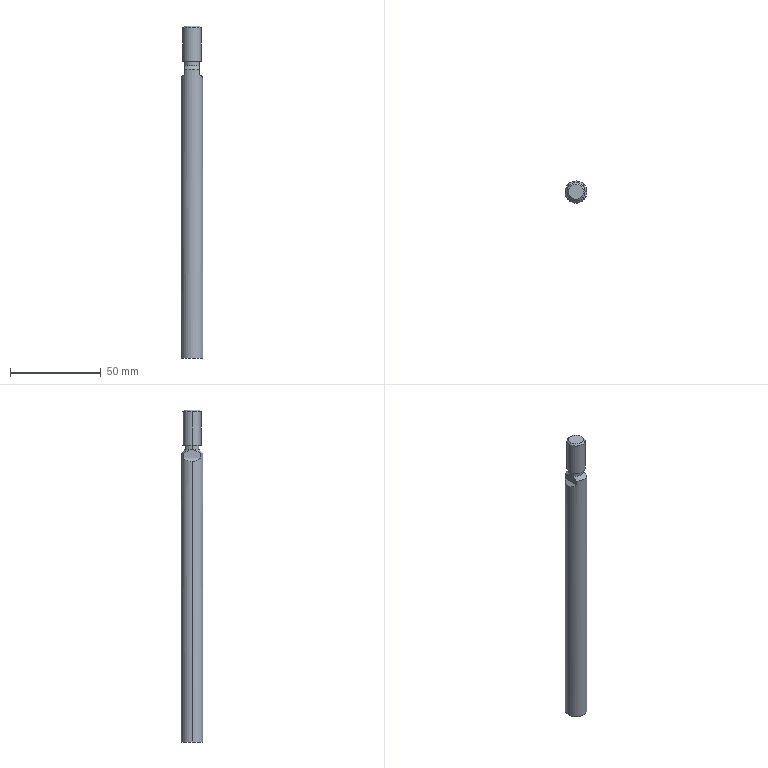Part | STEP file | rod_A_CDM2B32_150_C76_0_ | 1 solid | 19 faces | box 12 x 12 x 183 mm | volume 19693 mm3 | plane 9 | cylinder 6 | cone 4 | commonest cylinder face diameters 8.16 x2 10 x2 12 x2
STEP:
#1=CARTESIAN_POINT('',(6.,0.,-151.));
#2=VERTEX_POINT('',#1);
#3=CARTESIAN_POINT('',(-6.,0.,-151.));
#4=VERTEX_POINT('',#3);
#5=CARTESIAN_POINT('',(0.,0.,-151.));
#6=DIRECTION('',(0.,0.,1.));
#7=DIRECTION('',(1.,0.,0.));
#8=AXIS2_PLACEMENT_3D('',#5,#6,#7);
#9=CIRCLE('',#8,6.);
#10=EDGE_CURVE('',#2,#4,#9,.T.);
#11=ORIENTED_EDGE('',*,*,#10,.T.);
#12=CARTESIAN_POINT('',(-6.,0.,3.5));
#13=VERTEX_POINT('',#12);
#14=CARTESIAN_POINT('',(-6.,0.,-151.));
#15=DIRECTION('',(0.,0.,1.));
#16=VECTOR('',#15,1000.);
#17=LINE('',#14,#16);
#18=EDGE_CURVE('',#4,#13,#17,.T.);
#19=ORIENTED_EDGE('',*,*,#18,.T.);
#20=CARTESIAN_POINT('',(-4.,4.472,5.5));
#21=VERTEX_POINT('',#20);
#22=CARTESIAN_POINT('',(-6.,0.,3.5));
#23=CARTESIAN_POINT('',(-6.,1.734,3.5));
#24=CARTESIAN_POINT('',(-5.292,3.316,4.208));
#25=CARTESIAN_POINT('',(-4.,4.472,5.5));
#26=(BOUNDED_CURVE()B_SPLINE_CURVE(3,(#22,#23,#24,#25),.UNSPECIFIED.,.F.,.F.)B_SPLINE_CURVE_WITH_KNOTS((4,4),(3.142,3.983),.UNSPECIFIED.)CURVE()GEOMETRIC_REPRESENTATION_ITEM()RATIONAL_B_SPLINE_CURVE((1.,0.9419,0.9419,1.))REPRESENTATION_ITEM(''));
#27=EDGE_CURVE('',#13,#21,#26,.T.);
#28=ORIENTED_EDGE('',*,*,#27,.T.);
#29=CARTESIAN_POINT('',(-4.,4.472,8.08));
#30=VERTEX_POINT('',#29);
#31=CARTESIAN_POINT('',(-4.,4.472,-151.));
#32=DIRECTION('',(0.,0.,1.));
#33=VECTOR('',#32,1000.);
#34=LINE('',#31,#33);
#35=EDGE_CURVE('',#21,#30,#34,.T.);
#36=ORIENTED_EDGE('',*,*,#35,.T.);
#37=CARTESIAN_POINT('',(4.,4.472,8.08));
#38=VERTEX_POINT('',#37);
#39=CARTESIAN_POINT('',(0.,0.,8.08));
#40=DIRECTION('',(0.,0.,1.));
#41=DIRECTION('',(1.,0.,0.));
#42=AXIS2_PLACEMENT_3D('',#39,#40,#41);
#43=CIRCLE('',#42,6.);
#44=EDGE_CURVE('',#38,#30,#43,.T.);
#45=ORIENTED_EDGE('',*,*,#44,.F.);
#46=CARTESIAN_POINT('',(4.,4.472,5.5));
#47=VERTEX_POINT('',#46);
#48=CARTESIAN_POINT('',(4.,4.472,-151.));
#49=DIRECTION('',(0.,0.,-1.));
#50=VECTOR('',#49,1000.);
#51=LINE('',#48,#50);
#52=EDGE_CURVE('',#38,#47,#51,.T.);
#53=ORIENTED_EDGE('',*,*,#52,.T.);
#54=CARTESIAN_POINT('',(6.,0.,3.5));
#55=VERTEX_POINT('',#54);
#56=CARTESIAN_POINT('',(4.,4.472,5.5));
#57=CARTESIAN_POINT('',(5.292,3.316,4.208));
#58=CARTESIAN_POINT('',(6.,1.734,3.5));
#59=CARTESIAN_POINT('',(6.,0.,3.5));
#60=(BOUNDED_CURVE()B_SPLINE_CURVE(3,(#56,#57,#58,#59),.UNSPECIFIED.,.F.,.F.)B_SPLINE_CURVE_WITH_KNOTS((4,4),(2.301,3.142),.UNSPECIFIED.)CURVE()GEOMETRIC_REPRESENTATION_ITEM()RATIONAL_B_SPLINE_CURVE((1.,0.9419,0.9419,1.))REPRESENTATION_ITEM(''));
#61=EDGE_CURVE('',#47,#55,#60,.T.);
#62=ORIENTED_EDGE('',*,*,#61,.T.);
#63=CARTESIAN_POINT('',(6.,0.,-151.));
#64=DIRECTION('',(0.,0.,1.));
#65=VECTOR('',#64,1000.);
#66=LINE('',#63,#65);
#67=EDGE_CURVE('',#2,#55,#66,.T.);
#68=ORIENTED_EDGE('',*,*,#67,.F.);
#69=EDGE_LOOP('',(#11,#19,#28,#36,#45,#53,#62,#68));
#70=FACE_OUTER_BOUND('',#69,.T.);
#71=CARTESIAN_POINT('',(0.,0.,-151.));
#72=DIRECTION('',(0.,0.,1.));
#73=DIRECTION('',(1.,0.,0.));
#74=AXIS2_PLACEMENT_3D('',#71,#72,#73);
#75=CYLINDRICAL_SURFACE('',#74,6.);
#76=ADVANCED_FACE('',(#70),#75,.T.);
#77=CARTESIAN_POINT('',(-4.,0.804,10.));
#78=VERTEX_POINT('',#77);
#79=CARTESIAN_POINT('',(-4.08,0.,10.));
#80=VERTEX_POINT('',#79);
#81=CARTESIAN_POINT('',(0.,0.,10.));
#82=DIRECTION('',(0.,0.,1.));
#83=DIRECTION('',(1.,0.,0.));
#84=AXIS2_PLACEMENT_3D('',#81,#82,#83);
#85=CIRCLE('',#84,4.08);
#86=EDGE_CURVE('',#78,#80,#85,.T.);
#87=ORIENTED_EDGE('',*,*,#86,.T.);
#88=CARTESIAN_POINT('',(-4.08,0.,12.5));
#89=VERTEX_POINT('',#88);
#90=CARTESIAN_POINT('',(-4.08,0.,-151.));
#91=DIRECTION('',(0.,0.,1.));
#92=VECTOR('',#91,1000.);
#93=LINE('',#90,#92);
#94=EDGE_CURVE('',#80,#89,#93,.T.);
#95=ORIENTED_EDGE('',*,*,#94,.T.);
#96=CARTESIAN_POINT('',(4.08,0.,12.5));
#97=VERTEX_POINT('',#96);
#98=CARTESIAN_POINT('',(0.,0.,12.5));
#99=DIRECTION('',(0.,0.,1.));
#100=DIRECTION('',(1.,0.,0.));
#101=AXIS2_PLACEMENT_3D('',#98,#99,#100);
#102=CIRCLE('',#101,4.08);
#103=EDGE_CURVE('',#97,#89,#102,.T.);
#104=ORIENTED_EDGE('',*,*,#103,.F.);
#105=CARTESIAN_POINT('',(4.08,0.,10.));
#106=VERTEX_POINT('',#105);
#107=CARTESIAN_POINT('',(4.08,0.,-151.));
#108=DIRECTION('',(0.,0.,1.));
#109=VECTOR('',#108,1000.);
#110=LINE('',#107,#109);
#111=EDGE_CURVE('',#106,#97,#110,.T.);
#112=ORIENTED_EDGE('',*,*,#111,.F.);
#113=CARTESIAN_POINT('',(4.,0.804,10.));
#114=VERTEX_POINT('',#113);
#115=CARTESIAN_POINT('',(0.,0.,10.));
#116=DIRECTION('',(0.,0.,1.));
#117=DIRECTION('',(1.,0.,0.));
#118=AXIS2_PLACEMENT_3D('',#115,#116,#117);
#119=CIRCLE('',#118,4.08);
#120=EDGE_CURVE('',#106,#114,#119,.T.);
#121=ORIENTED_EDGE('',*,*,#120,.T.);
#122=CARTESIAN_POINT('',(0.,0.,10.));
#123=DIRECTION('',(0.,0.,1.));
#124=DIRECTION('',(1.,0.,0.));
#125=AXIS2_PLACEMENT_3D('',#122,#123,#124);
#126=CIRCLE('',#125,4.08);
#127=EDGE_CURVE('',#114,#78,#126,.T.);
#128=ORIENTED_EDGE('',*,*,#127,.T.);
#129=EDGE_LOOP('',(#87,#95,#104,#112,#121,#128));
#130=FACE_OUTER_BOUND('',#129,.T.);
#131=CARTESIAN_POINT('',(0.,0.,-151.));
#132=DIRECTION('',(0.,0.,1.));
#133=DIRECTION('',(1.,0.,0.));
#134=AXIS2_PLACEMENT_3D('',#131,#132,#133);
#135=CYLINDRICAL_SURFACE('',#134,4.08);
#136=ADVANCED_FACE('',(#130),#135,.T.);
#137=CARTESIAN_POINT('',(5.,0.,12.5));
#138=VERTEX_POINT('',#137);
#139=CARTESIAN_POINT('',(-5.,0.,12.5));
#140=VERTEX_POINT('',#139);
#141=CARTESIAN_POINT('',(0.,0.,12.5));
#142=DIRECTION('',(0.,0.,1.));
#143=DIRECTION('',(1.,0.,0.));
#144=AXIS2_PLACEMENT_3D('',#141,#142,#143);
#145=CIRCLE('',#144,5.);
#146=EDGE_CURVE('',#138,#140,#145,.T.);
#147=ORIENTED_EDGE('',*,*,#146,.T.);
#148=CARTESIAN_POINT('',(-5.,0.,31.08));
#149=VERTEX_POINT('',#148);
#150=CARTESIAN_POINT('',(-5.,0.,-151.));
#151=DIRECTION('',(0.,0.,1.));
#152=VECTOR('',#151,1000.);
#153=LINE('',#150,#152);
#154=EDGE_CURVE('',#140,#149,#153,.T.);
#155=ORIENTED_EDGE('',*,*,#154,.T.);
#156=CARTESIAN_POINT('',(5.,0.,31.08));
#157=VERTEX_POINT('',#156);
#158=CARTESIAN_POINT('',(0.,0.,31.08));
#159=DIRECTION('',(0.,0.,1.));
#160=DIRECTION('',(1.,0.,0.));
#161=AXIS2_PLACEMENT_3D('',#158,#159,#160);
#162=CIRCLE('',#161,5.);
#163=EDGE_CURVE('',#157,#149,#162,.T.);
#164=ORIENTED_EDGE('',*,*,#163,.F.);
#165=CARTESIAN_POINT('',(5.,0.,-151.));
#166=DIRECTION('',(0.,0.,1.));
#167=VECTOR('',#166,1000.);
#168=LINE('',#165,#167);
#169=EDGE_CURVE('',#138,#157,#168,.T.);
#170=ORIENTED_EDGE('',*,*,#169,.F.);
#171=EDGE_LOOP('',(#147,#155,#164,#170));
#172=FACE_OUTER_BOUND('',#171,.T.);
#173=CARTESIAN_POINT('',(0.,0.,-151.));
#174=DIRECTION('',(0.,0.,1.));
#175=DIRECTION('',(1.,0.,0.));
#176=AXIS2_PLACEMENT_3D('',#173,#174,#175);
#177=CYLINDRICAL_SURFACE('',#176,5.);
#178=ADVANCED_FACE('',(#172),#177,.T.);
#179=CARTESIAN_POINT('',(4.08,0.,32.));
#180=VERTEX_POINT('',#179);
#181=CARTESIAN_POINT('',(-4.08,0.,32.));
#182=VERTEX_POINT('',#181);
#183=CARTESIAN_POINT('',(0.,0.,32.));
#184=DIRECTION('',(0.,0.,1.));
#185=DIRECTION('',(1.,0.,0.));
#186=AXIS2_PLACEMENT_3D('',#183,#184,#185);
#187=CIRCLE('',#186,4.08);
#188=EDGE_CURVE('',#180,#182,#187,.T.);
#189=ORIENTED_EDGE('',*,*,#188,.F.);
#190=CARTESIAN_POINT('',(5.,0.,31.08));
#191=DIRECTION('',(0.7071,0.,-0.7071));
#192=VECTOR('',#191,1000.);
#193=LINE('',#190,#192);
#194=EDGE_CURVE('',#180,#157,#193,.T.);
#195=ORIENTED_EDGE('',*,*,#194,.T.);
#196=ORIENTED_EDGE('',*,*,#163,.T.);
#197=CARTESIAN_POINT('',(-5.,0.,31.08));
#198=DIRECTION('',(-0.7071,0.,-0.7071));
#199=VECTOR('',#198,1000.);
#200=LINE('',#197,#199);
#201=EDGE_CURVE('',#182,#149,#200,.T.);
#202=ORIENTED_EDGE('',*,*,#201,.F.);
#203=EDGE_LOOP('',(#189,#195,#196,#202));
#204=FACE_OUTER_BOUND('',#203,.T.);
#205=CARTESIAN_POINT('',(0.,0.,31.08));
#206=DIRECTION('',(0.,0.,-1.));
#207=DIRECTION('',(-1.,0.,0.));
#208=AXIS2_PLACEMENT_3D('',#205,#206,#207);
#209=CONICAL_SURFACE('',#208,5.,0.7854);
#210=ADVANCED_FACE('',(#204),#209,.T.);
#211=ORIENTED_EDGE('',*,*,#44,.T.);
#212=CARTESIAN_POINT('',(-4.,4.472,8.08));
#213=CARTESIAN_POINT('',(-4.,4.194,8.287));
#214=CARTESIAN_POINT('',(-4.,3.911,8.49));
#215=CARTESIAN_POINT('',(-4.,3.334,8.877));
#216=CARTESIAN_POINT('',(-4.,3.038,9.063));
#217=CARTESIAN_POINT('',(-4.,2.432,9.405));
#218=CARTESIAN_POINT('',(-4.,2.122,9.561));
#219=CARTESIAN_POINT('',(-4.,1.478,9.826));
#220=CARTESIAN_POINT('',(-4.,1.143,9.933));
#221=CARTESIAN_POINT('',(-4.,0.804,10.));
#222=B_SPLINE_CURVE_WITH_KNOTS('',3,(#212,#213,#214,#215,#216,#217,#218,#219,#220,#221),.UNSPECIFIED.,.F.,.F.,(4,2,2,2,4),(0.01098,0.01203,0.01307,0.01411,0.01515),.UNSPECIFIED.);
#223=EDGE_CURVE('',#30,#78,#222,.T.);
#224=ORIENTED_EDGE('',*,*,#223,.T.);
#225=ORIENTED_EDGE('',*,*,#127,.F.);
#226=CARTESIAN_POINT('',(4.,0.804,10.));
#227=CARTESIAN_POINT('',(4.,1.145,9.933));
#228=CARTESIAN_POINT('',(4.,1.483,9.824));
#229=CARTESIAN_POINT('',(4.,2.128,9.559));
#230=CARTESIAN_POINT('',(4.,2.437,9.403));
#231=CARTESIAN_POINT('',(4.,3.341,8.892));
#232=CARTESIAN_POINT('',(4.,3.914,8.496));
#233=CARTESIAN_POINT('',(4.,4.472,8.08));
#234=B_SPLINE_CURVE_WITH_KNOTS('',3,(#226,#227,#228,#229,#230,#231,#232,#233),.UNSPECIFIED.,.F.,.F.,(4,2,2,4),(0.01677,0.01782,0.01887,0.02097),.UNSPECIFIED.);
#235=EDGE_CURVE('',#114,#38,#234,.T.);
#236=ORIENTED_EDGE('',*,*,#235,.T.);
#237=EDGE_LOOP('',(#211,#224,#225,#236));
#238=FACE_OUTER_BOUND('',#237,.T.);
#239=CARTESIAN_POINT('',(0.,0.,8.08));
#240=DIRECTION('',(0.,0.,-1.));
#241=DIRECTION('',(-1.,0.,0.));
#242=AXIS2_PLACEMENT_3D('',#239,#240,#241);
#243=CONICAL_SURFACE('',#242,6.,0.7854);
#244=ADVANCED_FACE('',(#238),#243,.T.);
#245=CARTESIAN_POINT('',(0.,0.,32.));
#246=DIRECTION('',(0.,0.,1.));
#247=DIRECTION('',(1.,0.,0.));
#248=AXIS2_PLACEMENT_3D('',#245,#246,#247);
#249=CIRCLE('',#248,4.08);
#250=EDGE_CURVE('',#182,#180,#249,.T.);
#251=ORIENTED_EDGE('',*,*,#250,.T.);
#252=ORIENTED_EDGE('',*,*,#188,.T.);
#253=EDGE_LOOP('',(#251,#252));
#254=FACE_OUTER_BOUND('',#253,.T.);
#255=CARTESIAN_POINT('',(0.,0.,32.));
#256=DIRECTION('',(0.,0.,-1.));
#257=DIRECTION('',(-1.,0.,0.));
#258=AXIS2_PLACEMENT_3D('',#255,#256,#257);
#259=PLANE('',#258);
#260=ADVANCED_FACE('',(#254),#259,.F.);
#261=ORIENTED_EDGE('',*,*,#194,.F.);
#262=ORIENTED_EDGE('',*,*,#250,.F.);
#263=ORIENTED_EDGE('',*,*,#201,.T.);
#264=CARTESIAN_POINT('',(0.,0.,31.08));
#265=DIRECTION('',(0.,0.,1.));
#266=DIRECTION('',(1.,0.,0.));
#267=AXIS2_PLACEMENT_3D('',#264,#265,#266);
#268=CIRCLE('',#267,5.);
#269=EDGE_CURVE('',#149,#157,#268,.T.);
#270=ORIENTED_EDGE('',*,*,#269,.T.);
#271=EDGE_LOOP('',(#261,#262,#263,#270));
#272=FACE_OUTER_BOUND('',#271,.T.);
#273=CARTESIAN_POINT('',(0.,0.,31.08));
#274=DIRECTION('',(0.,0.,-1.));
#275=DIRECTION('',(-1.,0.,0.));
#276=AXIS2_PLACEMENT_3D('',#273,#274,#275);
#277=CONICAL_SURFACE('',#276,5.,0.7854);
#278=ADVANCED_FACE('',(#272),#277,.T.);
#279=ORIENTED_EDGE('',*,*,#154,.F.);
#280=CARTESIAN_POINT('',(0.,0.,12.5));
#281=DIRECTION('',(0.,0.,1.));
#282=DIRECTION('',(1.,0.,0.));
#283=AXIS2_PLACEMENT_3D('',#280,#281,#282);
#284=CIRCLE('',#283,5.);
#285=EDGE_CURVE('',#140,#138,#284,.T.);
#286=ORIENTED_EDGE('',*,*,#285,.T.);
#287=ORIENTED_EDGE('',*,*,#169,.T.);
#288=ORIENTED_EDGE('',*,*,#269,.F.);
#289=EDGE_LOOP('',(#279,#286,#287,#288));
#290=FACE_OUTER_BOUND('',#289,.T.);
#291=CARTESIAN_POINT('',(0.,0.,-151.));
#292=DIRECTION('',(0.,0.,1.));
#293=DIRECTION('',(1.,0.,0.));
#294=AXIS2_PLACEMENT_3D('',#291,#292,#293);
#295=CYLINDRICAL_SURFACE('',#294,5.);
#296=ADVANCED_FACE('',(#290),#295,.T.);
#297=ORIENTED_EDGE('',*,*,#146,.F.);
#298=ORIENTED_EDGE('',*,*,#285,.F.);
#299=EDGE_LOOP('',(#297,#298));
#300=FACE_OUTER_BOUND('',#299,.T.);
#301=ORIENTED_EDGE('',*,*,#103,.T.);
#302=CARTESIAN_POINT('',(0.,0.,12.5));
#303=DIRECTION('',(0.,0.,1.));
#304=DIRECTION('',(1.,0.,0.));
#305=AXIS2_PLACEMENT_3D('',#302,#303,#304);
#306=CIRCLE('',#305,4.08);
#307=EDGE_CURVE('',#89,#97,#306,.T.);
#308=ORIENTED_EDGE('',*,*,#307,.T.);
#309=EDGE_LOOP('',(#301,#308));
#310=FACE_BOUND('',#309,.T.);
#311=CARTESIAN_POINT('',(0.,5.,12.5));
#312=DIRECTION('',(0.,0.,1.));
#313=DIRECTION('',(1.,0.,0.));
#314=AXIS2_PLACEMENT_3D('',#311,#312,#313);
#315=PLANE('',#314);
#316=ADVANCED_FACE('',(#300,#310),#315,.F.);
#317=ORIENTED_EDGE('',*,*,#94,.F.);
#318=CARTESIAN_POINT('',(-4.,-0.804,10.));
#319=VERTEX_POINT('',#318);
#320=CARTESIAN_POINT('',(0.,0.,10.));
#321=DIRECTION('',(0.,0.,1.));
#322=DIRECTION('',(1.,0.,0.));
#323=AXIS2_PLACEMENT_3D('',#320,#321,#322);
#324=CIRCLE('',#323,4.08);
#325=EDGE_CURVE('',#80,#319,#324,.T.);
#326=ORIENTED_EDGE('',*,*,#325,.T.);
#327=CARTESIAN_POINT('',(4.,-0.804,10.));
#328=VERTEX_POINT('',#327);
#329=CARTESIAN_POINT('',(0.,0.,10.));
#330=DIRECTION('',(0.,0.,1.));
#331=DIRECTION('',(1.,0.,0.));
#332=AXIS2_PLACEMENT_3D('',#329,#330,#331);
#333=CIRCLE('',#332,4.08);
#334=EDGE_CURVE('',#319,#328,#333,.T.);
#335=ORIENTED_EDGE('',*,*,#334,.T.);
#336=CARTESIAN_POINT('',(0.,0.,10.));
#337=DIRECTION('',(0.,0.,1.));
#338=DIRECTION('',(1.,0.,0.));
#339=AXIS2_PLACEMENT_3D('',#336,#337,#338);
#340=CIRCLE('',#339,4.08);
#341=EDGE_CURVE('',#328,#106,#340,.T.);
#342=ORIENTED_EDGE('',*,*,#341,.T.);
#343=ORIENTED_EDGE('',*,*,#111,.T.);
#344=ORIENTED_EDGE('',*,*,#307,.F.);
#345=EDGE_LOOP('',(#317,#326,#335,#342,#343,#344));
#346=FACE_OUTER_BOUND('',#345,.T.);
#347=CARTESIAN_POINT('',(0.,0.,-151.));
#348=DIRECTION('',(0.,0.,1.));
#349=DIRECTION('',(1.,0.,0.));
#350=AXIS2_PLACEMENT_3D('',#347,#348,#349);
#351=CYLINDRICAL_SURFACE('',#350,4.08);
#352=ADVANCED_FACE('',(#346),#351,.T.);
#353=ORIENTED_EDGE('',*,*,#334,.F.);
#354=CARTESIAN_POINT('',(-4.,-4.472,8.08));
#355=VERTEX_POINT('',#354);
#356=CARTESIAN_POINT('',(-4.,-0.804,10.));
#357=CARTESIAN_POINT('',(-4.,-1.145,9.933));
#358=CARTESIAN_POINT('',(-4.,-1.483,9.824));
#359=CARTESIAN_POINT('',(-4.,-2.128,9.559));
#360=CARTESIAN_POINT('',(-4.,-2.437,9.403));
#361=CARTESIAN_POINT('',(-4.,-3.341,8.892));
#362=CARTESIAN_POINT('',(-4.,-3.914,8.496));
#363=CARTESIAN_POINT('',(-4.,-4.472,8.08));
#364=B_SPLINE_CURVE_WITH_KNOTS('',3,(#356,#357,#358,#359,#360,#361,#362,#363),.UNSPECIFIED.,.F.,.F.,(4,2,2,4),(0.01677,0.01782,0.01887,0.02097),.UNSPECIFIED.);
#365=EDGE_CURVE('',#319,#355,#364,.T.);
#366=ORIENTED_EDGE('',*,*,#365,.T.);
#367=CARTESIAN_POINT('',(4.,-4.472,8.08));
#368=VERTEX_POINT('',#367);
#369=CARTESIAN_POINT('',(0.,0.,8.08));
#370=DIRECTION('',(0.,0.,1.));
#371=DIRECTION('',(1.,0.,0.));
#372=AXIS2_PLACEMENT_3D('',#369,#370,#371);
#373=CIRCLE('',#372,6.);
#374=EDGE_CURVE('',#355,#368,#373,.T.);
#375=ORIENTED_EDGE('',*,*,#374,.T.);
#376=CARTESIAN_POINT('',(4.,-4.472,8.08));
#377=CARTESIAN_POINT('',(4.,-4.194,8.287));
#378=CARTESIAN_POINT('',(4.,-3.911,8.49));
#379=CARTESIAN_POINT('',(4.,-3.334,8.877));
#380=CARTESIAN_POINT('',(4.,-3.038,9.063));
#381=CARTESIAN_POINT('',(4.,-2.432,9.405));
#382=CARTESIAN_POINT('',(4.,-2.122,9.561));
#383=CARTESIAN_POINT('',(4.,-1.478,9.826));
#384=CARTESIAN_POINT('',(4.,-1.143,9.933));
#385=CARTESIAN_POINT('',(4.,-0.804,10.));
#386=B_SPLINE_CURVE_WITH_KNOTS('',3,(#376,#377,#378,#379,#380,#381,#382,#383,#384,#385),.UNSPECIFIED.,.F.,.F.,(4,2,2,2,4),(0.01098,0.01203,0.01307,0.01411,0.01515),.UNSPECIFIED.);
#387=EDGE_CURVE('',#368,#328,#386,.T.);
#388=ORIENTED_EDGE('',*,*,#387,.T.);
#389=EDGE_LOOP('',(#353,#366,#375,#388));
#390=FACE_OUTER_BOUND('',#389,.T.);
#391=CARTESIAN_POINT('',(0.,0.,8.08));
#392=DIRECTION('',(0.,0.,-1.));
#393=DIRECTION('',(-1.,0.,0.));
#394=AXIS2_PLACEMENT_3D('',#391,#392,#393);
#395=CONICAL_SURFACE('',#394,6.,0.7854);
#396=ADVANCED_FACE('',(#390),#395,.T.);
#397=ORIENTED_EDGE('',*,*,#18,.F.);
#398=CARTESIAN_POINT('',(0.,0.,-151.));
#399=DIRECTION('',(0.,0.,1.));
#400=DIRECTION('',(1.,0.,0.));
#401=AXIS2_PLACEMENT_3D('',#398,#399,#400);
#402=CIRCLE('',#401,6.);
#403=EDGE_CURVE('',#4,#2,#402,.T.);
#404=ORIENTED_EDGE('',*,*,#403,.T.);
#405=ORIENTED_EDGE('',*,*,#67,.T.);
#406=CARTESIAN_POINT('',(4.,-4.472,5.5));
#407=VERTEX_POINT('',#406);
#408=CARTESIAN_POINT('',(6.,0.,3.5));
#409=CARTESIAN_POINT('',(6.,-1.734,3.5));
#410=CARTESIAN_POINT('',(5.292,-3.316,4.208));
#411=CARTESIAN_POINT('',(4.,-4.472,5.5));
#412=(BOUNDED_CURVE()B_SPLINE_CURVE(3,(#408,#409,#410,#411),.UNSPECIFIED.,.F.,.T.)B_SPLINE_CURVE_WITH_KNOTS((4,4),(3.142,3.983),.UNSPECIFIED.)CURVE()GEOMETRIC_REPRESENTATION_ITEM()RATIONAL_B_SPLINE_CURVE((1.,0.9419,0.9419,1.))REPRESENTATION_ITEM(''));
#413=EDGE_CURVE('',#55,#407,#412,.T.);
#414=ORIENTED_EDGE('',*,*,#413,.T.);
#415=CARTESIAN_POINT('',(4.,-4.472,-151.));
#416=DIRECTION('',(0.,0.,1.));
#417=VECTOR('',#416,1000.);
#418=LINE('',#415,#417);
#419=EDGE_CURVE('',#407,#368,#418,.T.);
#420=ORIENTED_EDGE('',*,*,#419,.T.);
#421=ORIENTED_EDGE('',*,*,#374,.F.);
#422=CARTESIAN_POINT('',(-4.,-4.472,5.5));
#423=VERTEX_POINT('',#422);
#424=CARTESIAN_POINT('',(-4.,-4.472,-151.));
#425=DIRECTION('',(0.,0.,-1.));
#426=VECTOR('',#425,1000.);
#427=LINE('',#424,#426);
#428=EDGE_CURVE('',#355,#423,#427,.T.);
#429=ORIENTED_EDGE('',*,*,#428,.T.);
#430=CARTESIAN_POINT('',(-4.,-4.472,5.5));
#431=CARTESIAN_POINT('',(-5.292,-3.316,4.208));
#432=CARTESIAN_POINT('',(-6.,-1.734,3.5));
#433=CARTESIAN_POINT('',(-6.,0.,3.5));
#434=(BOUNDED_CURVE()B_SPLINE_CURVE(3,(#430,#431,#432,#433),.UNSPECIFIED.,.F.,.T.)B_SPLINE_CURVE_WITH_KNOTS((4,4),(2.301,3.142),.UNSPECIFIED.)CURVE()GEOMETRIC_REPRESENTATION_ITEM()RATIONAL_B_SPLINE_CURVE((1.,0.9419,0.9419,1.))REPRESENTATION_ITEM(''));
#435=EDGE_CURVE('',#423,#13,#434,.T.);
#436=ORIENTED_EDGE('',*,*,#435,.T.);
#437=EDGE_LOOP('',(#397,#404,#405,#414,#420,#421,#429,#436));
#438=FACE_OUTER_BOUND('',#437,.T.);
#439=CARTESIAN_POINT('',(0.,0.,-151.));
#440=DIRECTION('',(0.,0.,1.));
#441=DIRECTION('',(1.,0.,0.));
#442=AXIS2_PLACEMENT_3D('',#439,#440,#441);
#443=CYLINDRICAL_SURFACE('',#442,6.);
#444=ADVANCED_FACE('',(#438),#443,.T.);
#445=ORIENTED_EDGE('',*,*,#10,.F.);
#446=ORIENTED_EDGE('',*,*,#403,.F.);
#447=EDGE_LOOP('',(#445,#446));
#448=FACE_OUTER_BOUND('',#447,.T.);
#449=CARTESIAN_POINT('',(0.,6.,-151.));
#450=DIRECTION('',(0.,0.,1.));
#451=DIRECTION('',(1.,0.,0.));
#452=AXIS2_PLACEMENT_3D('',#449,#450,#451);
#453=PLANE('',#452);
#454=ADVANCED_FACE('',(#448),#453,.F.);
#455=CARTESIAN_POINT('',(4.,-12.,10.));
#456=DIRECTION('',(0.,1.,0.));
#457=VECTOR('',#456,1000.);
#458=LINE('',#455,#457);
#459=EDGE_CURVE('',#328,#114,#458,.T.);
#460=ORIENTED_EDGE('',*,*,#459,.T.);
#461=ORIENTED_EDGE('',*,*,#120,.F.);
#462=ORIENTED_EDGE('',*,*,#341,.F.);
#463=EDGE_LOOP('',(#460,#461,#462));
#464=FACE_OUTER_BOUND('',#463,.T.);
#465=CARTESIAN_POINT('',(4.,-12.,10.));
#466=DIRECTION('',(0.,0.,1.));
#467=DIRECTION('',(1.,0.,0.));
#468=AXIS2_PLACEMENT_3D('',#465,#466,#467);
#469=PLANE('',#468);
#470=ADVANCED_FACE('',(#464),#469,.F.);
#471=ORIENTED_EDGE('',*,*,#419,.F.);
#472=CARTESIAN_POINT('',(4.,-12.,5.5));
#473=DIRECTION('',(0.,1.,0.));
#474=VECTOR('',#473,1000.);
#475=LINE('',#472,#474);
#476=EDGE_CURVE('',#407,#47,#475,.T.);
#477=ORIENTED_EDGE('',*,*,#476,.T.);
#478=ORIENTED_EDGE('',*,*,#52,.F.);
#479=ORIENTED_EDGE('',*,*,#235,.F.);
#480=ORIENTED_EDGE('',*,*,#459,.F.);
#481=ORIENTED_EDGE('',*,*,#387,.F.);
#482=EDGE_LOOP('',(#471,#477,#478,#479,#480,#481));
#483=FACE_OUTER_BOUND('',#482,.T.);
#484=CARTESIAN_POINT('',(4.,-12.,5.5));
#485=DIRECTION('',(-1.,0.,0.));
#486=DIRECTION('',(0.,0.,1.));
#487=AXIS2_PLACEMENT_3D('',#484,#485,#486);
#488=PLANE('',#487);
#489=ADVANCED_FACE('',(#483),#488,.F.);
#490=ORIENTED_EDGE('',*,*,#476,.F.);
#491=ORIENTED_EDGE('',*,*,#413,.F.);
#492=ORIENTED_EDGE('',*,*,#61,.F.);
#493=EDGE_LOOP('',(#490,#491,#492));
#494=FACE_OUTER_BOUND('',#493,.T.);
#495=CARTESIAN_POINT('',(6.,-12.,3.5));
#496=DIRECTION('',(-0.7071,0.,-0.7071));
#497=DIRECTION('',(-0.7071,0.,0.7071));
#498=AXIS2_PLACEMENT_3D('',#495,#496,#497);
#499=PLANE('',#498);
#500=ADVANCED_FACE('',(#494),#499,.F.);
#501=CARTESIAN_POINT('',(-4.,-12.,10.));
#502=DIRECTION('',(0.,1.,0.));
#503=VECTOR('',#502,1000.);
#504=LINE('',#501,#503);
#505=EDGE_CURVE('',#319,#78,#504,.T.);
#506=ORIENTED_EDGE('',*,*,#505,.F.);
#507=ORIENTED_EDGE('',*,*,#325,.F.);
#508=ORIENTED_EDGE('',*,*,#86,.F.);
#509=EDGE_LOOP('',(#506,#507,#508));
#510=FACE_OUTER_BOUND('',#509,.T.);
#511=CARTESIAN_POINT('',(-8.,-12.,10.));
#512=DIRECTION('',(0.,0.,1.));
#513=DIRECTION('',(1.,0.,0.));
#514=AXIS2_PLACEMENT_3D('',#511,#512,#513);
#515=PLANE('',#514);
#516=ADVANCED_FACE('',(#510),#515,.F.);
#517=CARTESIAN_POINT('',(-4.,-12.,5.5));
#518=DIRECTION('',(0.,1.,0.));
#519=VECTOR('',#518,1000.);
#520=LINE('',#517,#519);
#521=EDGE_CURVE('',#423,#21,#520,.T.);
#522=ORIENTED_EDGE('',*,*,#521,.T.);
#523=ORIENTED_EDGE('',*,*,#27,.F.);
#524=ORIENTED_EDGE('',*,*,#435,.F.);
#525=EDGE_LOOP('',(#522,#523,#524));
#526=FACE_OUTER_BOUND('',#525,.T.);
#527=CARTESIAN_POINT('',(-4.,-12.,5.5));
#528=DIRECTION('',(0.7071,0.,-0.7071));
#529=DIRECTION('',(-0.7071,0.,-0.7071));
#530=AXIS2_PLACEMENT_3D('',#527,#528,#529);
#531=PLANE('',#530);
#532=ADVANCED_FACE('',(#526),#531,.F.);
#533=ORIENTED_EDGE('',*,*,#35,.F.);
#534=ORIENTED_EDGE('',*,*,#521,.F.);
#535=ORIENTED_EDGE('',*,*,#428,.F.);
#536=ORIENTED_EDGE('',*,*,#365,.F.);
#537=ORIENTED_EDGE('',*,*,#505,.T.);
#538=ORIENTED_EDGE('',*,*,#223,.F.);
#539=EDGE_LOOP('',(#533,#534,#535,#536,#537,#538));
#540=FACE_OUTER_BOUND('',#539,.T.);
#541=CARTESIAN_POINT('',(-4.,-12.,10.));
#542=DIRECTION('',(1.,0.,0.));
#543=DIRECTION('',(0.,0.,-1.));
#544=AXIS2_PLACEMENT_3D('',#541,#542,#543);
#545=PLANE('',#544);
#546=ADVANCED_FACE('',(#540),#545,.F.);
#547=CLOSED_SHELL('',(#76,#136,#178,#210,#244,#260,#278,#296,#316,#352,#396,#444,#454,#470,#489,#500,#516,#532,#546));
#548=MANIFOLD_SOLID_BREP('',#547);
#549=CARTESIAN_POINT('',(0.,0.,0.));
#550=DIRECTION('',(0.,0.,1.));
#551=DIRECTION('',(1.,0.,0.));
#552=AXIS2_PLACEMENT_3D('',#549,#550,#551);
#553=(LENGTH_UNIT()NAMED_UNIT(*)SI_UNIT(.MILLI.,.METRE.));
#554=UNCERTAINTY_MEASURE_WITH_UNIT(LENGTH_MEASURE(0.00001),#553,'','');
#555=(NAMED_UNIT(*)PLANE_ANGLE_UNIT()SI_UNIT($,.RADIAN.));
#556=(NAMED_UNIT(*)SI_UNIT($,.STERADIAN.)SOLID_ANGLE_UNIT());
#557=(GEOMETRIC_REPRESENTATION_CONTEXT(3)GLOBAL_UNCERTAINTY_ASSIGNED_CONTEXT((#554))GLOBAL_UNIT_ASSIGNED_CONTEXT((#553,#555,#556))REPRESENTATION_CONTEXT('',''));
#558=ADVANCED_BREP_SHAPE_REPRESENTATION('',(#548,#552),#557);